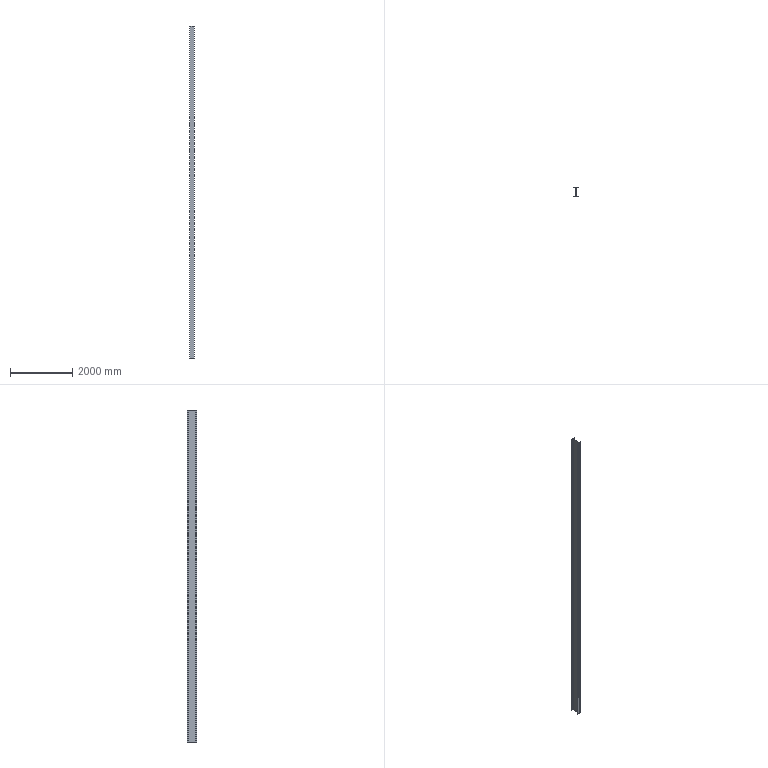Part | SolidWorks | features Extrusion 1 | 1 solid | 18 faces | box 150 x 300 x 10687 mm | volume 49994543 mm3 | plane 14 | cylinder 4 | commonest cylinder face diameters 26 x4
STEP:
#1=CARTESIAN_POINT('',(-75.,9.,0.));
#2=VERTEX_POINT('',#1);
#3=CARTESIAN_POINT('',(-75.,0.,0.));
#4=VERTEX_POINT('',#3);
#5=CARTESIAN_POINT('',(-75.,0.,0.));
#6=DIRECTION('',(0.,-1.,0.));
#7=VECTOR('',#6,1000.);
#8=LINE('',#5,#7);
#9=EDGE_CURVE('',#2,#4,#8,.T.);
#10=ORIENTED_EDGE('',*,*,#9,.T.);
#11=CARTESIAN_POINT('',(-75.,0.,10687.));
#12=VERTEX_POINT('',#11);
#13=CARTESIAN_POINT('',(-75.,0.,10687.));
#14=DIRECTION('',(0.,0.,-1.));
#15=VECTOR('',#14,1000.);
#16=LINE('',#13,#15);
#17=EDGE_CURVE('',#12,#4,#16,.T.);
#18=ORIENTED_EDGE('',*,*,#17,.F.);
#19=CARTESIAN_POINT('',(-75.,9.,10687.));
#20=VERTEX_POINT('',#19);
#21=CARTESIAN_POINT('',(-75.,0.,10687.));
#22=DIRECTION('',(0.,-1.,0.));
#23=VECTOR('',#22,1000.);
#24=LINE('',#21,#23);
#25=EDGE_CURVE('',#20,#12,#24,.T.);
#26=ORIENTED_EDGE('',*,*,#25,.F.);
#27=CARTESIAN_POINT('',(-75.,9.,10687.));
#28=DIRECTION('',(0.,0.,-1.));
#29=VECTOR('',#28,1000.);
#30=LINE('',#27,#29);
#31=EDGE_CURVE('',#20,#2,#30,.T.);
#32=ORIENTED_EDGE('',*,*,#31,.T.);
#33=EDGE_LOOP('',(#10,#18,#26,#32));
#34=FACE_OUTER_BOUND('',#33,.T.);
#35=CARTESIAN_POINT('',(-75.,0.,10687.));
#36=DIRECTION('',(1.,0.,0.));
#37=DIRECTION('',(0.,0.,-1.));
#38=AXIS2_PLACEMENT_3D('',#35,#36,#37);
#39=PLANE('',#38);
#40=ADVANCED_FACE('',(#34),#39,.F.);
#41=CARTESIAN_POINT('',(75.,0.,0.));
#42=VERTEX_POINT('',#41);
#43=CARTESIAN_POINT('',(75.,0.,0.));
#44=DIRECTION('',(1.,0.,0.));
#45=VECTOR('',#44,1000.);
#46=LINE('',#43,#45);
#47=EDGE_CURVE('',#4,#42,#46,.T.);
#48=ORIENTED_EDGE('',*,*,#47,.T.);
#49=CARTESIAN_POINT('',(75.,0.,10687.));
#50=VERTEX_POINT('',#49);
#51=CARTESIAN_POINT('',(75.,0.,10687.));
#52=DIRECTION('',(0.,0.,-1.));
#53=VECTOR('',#52,1000.);
#54=LINE('',#51,#53);
#55=EDGE_CURVE('',#50,#42,#54,.T.);
#56=ORIENTED_EDGE('',*,*,#55,.F.);
#57=CARTESIAN_POINT('',(75.,0.,10687.));
#58=DIRECTION('',(1.,0.,0.));
#59=VECTOR('',#58,1000.);
#60=LINE('',#57,#59);
#61=EDGE_CURVE('',#12,#50,#60,.T.);
#62=ORIENTED_EDGE('',*,*,#61,.F.);
#63=ORIENTED_EDGE('',*,*,#17,.T.);
#64=EDGE_LOOP('',(#48,#56,#62,#63));
#65=FACE_OUTER_BOUND('',#64,.T.);
#66=CARTESIAN_POINT('',(75.,0.,10687.));
#67=DIRECTION('',(0.,1.,0.));
#68=DIRECTION('',(-1.,0.,0.));
#69=AXIS2_PLACEMENT_3D('',#66,#67,#68);
#70=PLANE('',#69);
#71=ADVANCED_FACE('',(#65),#70,.F.);
#72=CARTESIAN_POINT('',(75.,9.,0.));
#73=VERTEX_POINT('',#72);
#74=CARTESIAN_POINT('',(75.,0.,0.));
#75=DIRECTION('',(0.,1.,0.));
#76=VECTOR('',#75,1000.);
#77=LINE('',#74,#76);
#78=EDGE_CURVE('',#42,#73,#77,.T.);
#79=ORIENTED_EDGE('',*,*,#78,.T.);
#80=CARTESIAN_POINT('',(75.,9.,10687.));
#81=VERTEX_POINT('',#80);
#82=CARTESIAN_POINT('',(75.,9.,10687.));
#83=DIRECTION('',(0.,0.,-1.));
#84=VECTOR('',#83,1000.);
#85=LINE('',#82,#84);
#86=EDGE_CURVE('',#81,#73,#85,.T.);
#87=ORIENTED_EDGE('',*,*,#86,.F.);
#88=CARTESIAN_POINT('',(75.,0.,10687.));
#89=DIRECTION('',(0.,1.,0.));
#90=VECTOR('',#89,1000.);
#91=LINE('',#88,#90);
#92=EDGE_CURVE('',#50,#81,#91,.T.);
#93=ORIENTED_EDGE('',*,*,#92,.F.);
#94=ORIENTED_EDGE('',*,*,#55,.T.);
#95=EDGE_LOOP('',(#79,#87,#93,#94));
#96=FACE_OUTER_BOUND('',#95,.T.);
#97=CARTESIAN_POINT('',(75.,0.,10687.));
#98=DIRECTION('',(-1.,0.,0.));
#99=DIRECTION('',(0.,0.,1.));
#100=AXIS2_PLACEMENT_3D('',#97,#98,#99);
#101=PLANE('',#100);
#102=ADVANCED_FACE('',(#96),#101,.F.);
#103=CARTESIAN_POINT('',(16.25,9.,0.));
#104=VERTEX_POINT('',#103);
#105=CARTESIAN_POINT('',(75.,9.,0.));
#106=DIRECTION('',(-1.,0.,0.));
#107=VECTOR('',#106,1000.);
#108=LINE('',#105,#107);
#109=EDGE_CURVE('',#73,#104,#108,.T.);
#110=ORIENTED_EDGE('',*,*,#109,.T.);
#111=CARTESIAN_POINT('',(16.25,9.,10687.));
#112=VERTEX_POINT('',#111);
#113=CARTESIAN_POINT('',(16.25,9.,10687.));
#114=DIRECTION('',(0.,0.,-1.));
#115=VECTOR('',#114,1000.);
#116=LINE('',#113,#115);
#117=EDGE_CURVE('',#112,#104,#116,.T.);
#118=ORIENTED_EDGE('',*,*,#117,.F.);
#119=CARTESIAN_POINT('',(75.,9.,10687.));
#120=DIRECTION('',(-1.,0.,0.));
#121=VECTOR('',#120,1000.);
#122=LINE('',#119,#121);
#123=EDGE_CURVE('',#81,#112,#122,.T.);
#124=ORIENTED_EDGE('',*,*,#123,.F.);
#125=ORIENTED_EDGE('',*,*,#86,.T.);
#126=EDGE_LOOP('',(#110,#118,#124,#125));
#127=FACE_OUTER_BOUND('',#126,.T.);
#128=CARTESIAN_POINT('',(75.,9.,10687.));
#129=DIRECTION('',(0.,-1.,0.));
#130=DIRECTION('',(1.,0.,0.));
#131=AXIS2_PLACEMENT_3D('',#128,#129,#130);
#132=PLANE('',#131);
#133=ADVANCED_FACE('',(#127),#132,.F.);
#134=CARTESIAN_POINT('',(3.25,22.,0.));
#135=VERTEX_POINT('',#134);
#136=CARTESIAN_POINT('',(16.25,22.,0.));
#137=DIRECTION('',(0.,0.,-1.));
#138=DIRECTION('',(-1.,0.,0.));
#139=AXIS2_PLACEMENT_3D('',#136,#137,#138);
#140=CIRCLE('',#139,13.);
#141=EDGE_CURVE('',#104,#135,#140,.T.);
#142=ORIENTED_EDGE('',*,*,#141,.T.);
#143=CARTESIAN_POINT('',(3.25,22.,10687.));
#144=VERTEX_POINT('',#143);
#145=CARTESIAN_POINT('',(3.25,22.,10687.));
#146=DIRECTION('',(0.,0.,-1.));
#147=VECTOR('',#146,1000.);
#148=LINE('',#145,#147);
#149=EDGE_CURVE('',#144,#135,#148,.T.);
#150=ORIENTED_EDGE('',*,*,#149,.F.);
#151=CARTESIAN_POINT('',(16.25,22.,10687.));
#152=DIRECTION('',(0.,0.,-1.));
#153=DIRECTION('',(-1.,0.,0.));
#154=AXIS2_PLACEMENT_3D('',#151,#152,#153);
#155=CIRCLE('',#154,13.);
#156=EDGE_CURVE('',#112,#144,#155,.T.);
#157=ORIENTED_EDGE('',*,*,#156,.F.);
#158=ORIENTED_EDGE('',*,*,#117,.T.);
#159=EDGE_LOOP('',(#142,#150,#157,#158));
#160=FACE_OUTER_BOUND('',#159,.T.);
#161=CARTESIAN_POINT('',(16.25,22.,10687.));
#162=DIRECTION('',(0.,0.,-1.));
#163=DIRECTION('',(-1.,0.,0.));
#164=AXIS2_PLACEMENT_3D('',#161,#162,#163);
#165=CYLINDRICAL_SURFACE('',#164,13.);
#166=ADVANCED_FACE('',(#160),#165,.F.);
#167=CARTESIAN_POINT('',(3.25,278.,0.));
#168=VERTEX_POINT('',#167);
#169=CARTESIAN_POINT('',(3.25,22.,0.));
#170=DIRECTION('',(0.,1.,0.));
#171=VECTOR('',#170,1000.);
#172=LINE('',#169,#171);
#173=EDGE_CURVE('',#135,#168,#172,.T.);
#174=ORIENTED_EDGE('',*,*,#173,.T.);
#175=CARTESIAN_POINT('',(3.25,278.,10687.));
#176=VERTEX_POINT('',#175);
#177=CARTESIAN_POINT('',(3.25,278.,10687.));
#178=DIRECTION('',(0.,0.,-1.));
#179=VECTOR('',#178,1000.);
#180=LINE('',#177,#179);
#181=EDGE_CURVE('',#176,#168,#180,.T.);
#182=ORIENTED_EDGE('',*,*,#181,.F.);
#183=CARTESIAN_POINT('',(3.25,22.,10687.));
#184=DIRECTION('',(0.,1.,0.));
#185=VECTOR('',#184,1000.);
#186=LINE('',#183,#185);
#187=EDGE_CURVE('',#144,#176,#186,.T.);
#188=ORIENTED_EDGE('',*,*,#187,.F.);
#189=ORIENTED_EDGE('',*,*,#149,.T.);
#190=EDGE_LOOP('',(#174,#182,#188,#189));
#191=FACE_OUTER_BOUND('',#190,.T.);
#192=CARTESIAN_POINT('',(3.25,22.,10687.));
#193=DIRECTION('',(-1.,0.,0.));
#194=DIRECTION('',(0.,0.,1.));
#195=AXIS2_PLACEMENT_3D('',#192,#193,#194);
#196=PLANE('',#195);
#197=ADVANCED_FACE('',(#191),#196,.F.);
#198=CARTESIAN_POINT('',(16.25,291.,0.));
#199=VERTEX_POINT('',#198);
#200=CARTESIAN_POINT('',(16.25,278.,0.));
#201=DIRECTION('',(0.,0.,-1.));
#202=DIRECTION('',(-1.,0.,0.));
#203=AXIS2_PLACEMENT_3D('',#200,#201,#202);
#204=CIRCLE('',#203,13.);
#205=EDGE_CURVE('',#168,#199,#204,.T.);
#206=ORIENTED_EDGE('',*,*,#205,.T.);
#207=CARTESIAN_POINT('',(16.25,291.,10687.));
#208=VERTEX_POINT('',#207);
#209=CARTESIAN_POINT('',(16.25,291.,10687.));
#210=DIRECTION('',(0.,0.,-1.));
#211=VECTOR('',#210,1000.);
#212=LINE('',#209,#211);
#213=EDGE_CURVE('',#208,#199,#212,.T.);
#214=ORIENTED_EDGE('',*,*,#213,.F.);
#215=CARTESIAN_POINT('',(16.25,278.,10687.));
#216=DIRECTION('',(0.,0.,-1.));
#217=DIRECTION('',(-1.,0.,0.));
#218=AXIS2_PLACEMENT_3D('',#215,#216,#217);
#219=CIRCLE('',#218,13.);
#220=EDGE_CURVE('',#176,#208,#219,.T.);
#221=ORIENTED_EDGE('',*,*,#220,.F.);
#222=ORIENTED_EDGE('',*,*,#181,.T.);
#223=EDGE_LOOP('',(#206,#214,#221,#222));
#224=FACE_OUTER_BOUND('',#223,.T.);
#225=CARTESIAN_POINT('',(16.25,278.,10687.));
#226=DIRECTION('',(0.,0.,-1.));
#227=DIRECTION('',(-1.,0.,0.));
#228=AXIS2_PLACEMENT_3D('',#225,#226,#227);
#229=CYLINDRICAL_SURFACE('',#228,13.);
#230=ADVANCED_FACE('',(#224),#229,.F.);
#231=CARTESIAN_POINT('',(75.,291.,0.));
#232=VERTEX_POINT('',#231);
#233=CARTESIAN_POINT('',(16.25,291.,0.));
#234=DIRECTION('',(1.,0.,0.));
#235=VECTOR('',#234,1000.);
#236=LINE('',#233,#235);
#237=EDGE_CURVE('',#199,#232,#236,.T.);
#238=ORIENTED_EDGE('',*,*,#237,.T.);
#239=CARTESIAN_POINT('',(75.,291.,10687.));
#240=VERTEX_POINT('',#239);
#241=CARTESIAN_POINT('',(75.,291.,10687.));
#242=DIRECTION('',(0.,0.,-1.));
#243=VECTOR('',#242,1000.);
#244=LINE('',#241,#243);
#245=EDGE_CURVE('',#240,#232,#244,.T.);
#246=ORIENTED_EDGE('',*,*,#245,.F.);
#247=CARTESIAN_POINT('',(16.25,291.,10687.));
#248=DIRECTION('',(1.,0.,0.));
#249=VECTOR('',#248,1000.);
#250=LINE('',#247,#249);
#251=EDGE_CURVE('',#208,#240,#250,.T.);
#252=ORIENTED_EDGE('',*,*,#251,.F.);
#253=ORIENTED_EDGE('',*,*,#213,.T.);
#254=EDGE_LOOP('',(#238,#246,#252,#253));
#255=FACE_OUTER_BOUND('',#254,.T.);
#256=CARTESIAN_POINT('',(16.25,291.,10687.));
#257=DIRECTION('',(0.,1.,0.));
#258=DIRECTION('',(-1.,0.,0.));
#259=AXIS2_PLACEMENT_3D('',#256,#257,#258);
#260=PLANE('',#259);
#261=ADVANCED_FACE('',(#255),#260,.F.);
#262=CARTESIAN_POINT('',(75.,300.,0.));
#263=VERTEX_POINT('',#262);
#264=CARTESIAN_POINT('',(75.,291.,0.));
#265=DIRECTION('',(0.,1.,0.));
#266=VECTOR('',#265,1000.);
#267=LINE('',#264,#266);
#268=EDGE_CURVE('',#232,#263,#267,.T.);
#269=ORIENTED_EDGE('',*,*,#268,.T.);
#270=CARTESIAN_POINT('',(75.,300.,10687.));
#271=VERTEX_POINT('',#270);
#272=CARTESIAN_POINT('',(75.,300.,10687.));
#273=DIRECTION('',(0.,0.,-1.));
#274=VECTOR('',#273,1000.);
#275=LINE('',#272,#274);
#276=EDGE_CURVE('',#271,#263,#275,.T.);
#277=ORIENTED_EDGE('',*,*,#276,.F.);
#278=CARTESIAN_POINT('',(75.,291.,10687.));
#279=DIRECTION('',(0.,1.,0.));
#280=VECTOR('',#279,1000.);
#281=LINE('',#278,#280);
#282=EDGE_CURVE('',#240,#271,#281,.T.);
#283=ORIENTED_EDGE('',*,*,#282,.F.);
#284=ORIENTED_EDGE('',*,*,#245,.T.);
#285=EDGE_LOOP('',(#269,#277,#283,#284));
#286=FACE_OUTER_BOUND('',#285,.T.);
#287=CARTESIAN_POINT('',(75.,291.,10687.));
#288=DIRECTION('',(-1.,0.,0.));
#289=DIRECTION('',(0.,-1.,0.));
#290=AXIS2_PLACEMENT_3D('',#287,#288,#289);
#291=PLANE('',#290);
#292=ADVANCED_FACE('',(#286),#291,.F.);
#293=CARTESIAN_POINT('',(-75.,300.,0.));
#294=VERTEX_POINT('',#293);
#295=CARTESIAN_POINT('',(-75.,300.,0.));
#296=DIRECTION('',(-1.,0.,0.));
#297=VECTOR('',#296,1000.);
#298=LINE('',#295,#297);
#299=EDGE_CURVE('',#263,#294,#298,.T.);
#300=ORIENTED_EDGE('',*,*,#299,.T.);
#301=CARTESIAN_POINT('',(-75.,300.,10687.));
#302=VERTEX_POINT('',#301);
#303=CARTESIAN_POINT('',(-75.,300.,10687.));
#304=DIRECTION('',(0.,0.,-1.));
#305=VECTOR('',#304,1000.);
#306=LINE('',#303,#305);
#307=EDGE_CURVE('',#302,#294,#306,.T.);
#308=ORIENTED_EDGE('',*,*,#307,.F.);
#309=CARTESIAN_POINT('',(-75.,300.,10687.));
#310=DIRECTION('',(-1.,0.,0.));
#311=VECTOR('',#310,1000.);
#312=LINE('',#309,#311);
#313=EDGE_CURVE('',#271,#302,#312,.T.);
#314=ORIENTED_EDGE('',*,*,#313,.F.);
#315=ORIENTED_EDGE('',*,*,#276,.T.);
#316=EDGE_LOOP('',(#300,#308,#314,#315));
#317=FACE_OUTER_BOUND('',#316,.T.);
#318=CARTESIAN_POINT('',(-75.,300.,10687.));
#319=DIRECTION('',(0.,-1.,0.));
#320=DIRECTION('',(0.,0.,-1.));
#321=AXIS2_PLACEMENT_3D('',#318,#319,#320);
#322=PLANE('',#321);
#323=ADVANCED_FACE('',(#317),#322,.F.);
#324=CARTESIAN_POINT('',(-75.,291.,0.));
#325=VERTEX_POINT('',#324);
#326=CARTESIAN_POINT('',(-75.,291.,0.));
#327=DIRECTION('',(0.,-1.,0.));
#328=VECTOR('',#327,1000.);
#329=LINE('',#326,#328);
#330=EDGE_CURVE('',#294,#325,#329,.T.);
#331=ORIENTED_EDGE('',*,*,#330,.T.);
#332=CARTESIAN_POINT('',(-75.,291.,10687.));
#333=VERTEX_POINT('',#332);
#334=CARTESIAN_POINT('',(-75.,291.,10687.));
#335=DIRECTION('',(0.,0.,-1.));
#336=VECTOR('',#335,1000.);
#337=LINE('',#334,#336);
#338=EDGE_CURVE('',#333,#325,#337,.T.);
#339=ORIENTED_EDGE('',*,*,#338,.F.);
#340=CARTESIAN_POINT('',(-75.,291.,10687.));
#341=DIRECTION('',(0.,-1.,0.));
#342=VECTOR('',#341,1000.);
#343=LINE('',#340,#342);
#344=EDGE_CURVE('',#302,#333,#343,.T.);
#345=ORIENTED_EDGE('',*,*,#344,.F.);
#346=ORIENTED_EDGE('',*,*,#307,.T.);
#347=EDGE_LOOP('',(#331,#339,#345,#346));
#348=FACE_OUTER_BOUND('',#347,.T.);
#349=CARTESIAN_POINT('',(-75.,291.,10687.));
#350=DIRECTION('',(1.,0.,0.));
#351=DIRECTION('',(0.,1.,0.));
#352=AXIS2_PLACEMENT_3D('',#349,#350,#351);
#353=PLANE('',#352);
#354=ADVANCED_FACE('',(#348),#353,.F.);
#355=CARTESIAN_POINT('',(-16.25,291.,0.));
#356=VERTEX_POINT('',#355);
#357=CARTESIAN_POINT('',(-16.25,291.,0.));
#358=DIRECTION('',(1.,0.,0.));
#359=VECTOR('',#358,1000.);
#360=LINE('',#357,#359);
#361=EDGE_CURVE('',#325,#356,#360,.T.);
#362=ORIENTED_EDGE('',*,*,#361,.T.);
#363=CARTESIAN_POINT('',(-16.25,291.,10687.));
#364=VERTEX_POINT('',#363);
#365=CARTESIAN_POINT('',(-16.25,291.,10687.));
#366=DIRECTION('',(0.,0.,-1.));
#367=VECTOR('',#366,1000.);
#368=LINE('',#365,#367);
#369=EDGE_CURVE('',#364,#356,#368,.T.);
#370=ORIENTED_EDGE('',*,*,#369,.F.);
#371=CARTESIAN_POINT('',(-16.25,291.,10687.));
#372=DIRECTION('',(1.,0.,0.));
#373=VECTOR('',#372,1000.);
#374=LINE('',#371,#373);
#375=EDGE_CURVE('',#333,#364,#374,.T.);
#376=ORIENTED_EDGE('',*,*,#375,.F.);
#377=ORIENTED_EDGE('',*,*,#338,.T.);
#378=EDGE_LOOP('',(#362,#370,#376,#377));
#379=FACE_OUTER_BOUND('',#378,.T.);
#380=CARTESIAN_POINT('',(-16.25,291.,10687.));
#381=DIRECTION('',(0.,1.,0.));
#382=DIRECTION('',(-1.,0.,0.));
#383=AXIS2_PLACEMENT_3D('',#380,#381,#382);
#384=PLANE('',#383);
#385=ADVANCED_FACE('',(#379),#384,.F.);
#386=CARTESIAN_POINT('',(-3.25,278.,0.));
#387=VERTEX_POINT('',#386);
#388=CARTESIAN_POINT('',(-16.25,278.,0.));
#389=DIRECTION('',(0.,0.,-1.));
#390=DIRECTION('',(1.,0.,0.));
#391=AXIS2_PLACEMENT_3D('',#388,#389,#390);
#392=CIRCLE('',#391,13.);
#393=EDGE_CURVE('',#356,#387,#392,.T.);
#394=ORIENTED_EDGE('',*,*,#393,.T.);
#395=CARTESIAN_POINT('',(-3.25,278.,10687.));
#396=VERTEX_POINT('',#395);
#397=CARTESIAN_POINT('',(-3.25,278.,10687.));
#398=DIRECTION('',(0.,0.,-1.));
#399=VECTOR('',#398,1000.);
#400=LINE('',#397,#399);
#401=EDGE_CURVE('',#396,#387,#400,.T.);
#402=ORIENTED_EDGE('',*,*,#401,.F.);
#403=CARTESIAN_POINT('',(-16.25,278.,10687.));
#404=DIRECTION('',(0.,0.,-1.));
#405=DIRECTION('',(1.,0.,0.));
#406=AXIS2_PLACEMENT_3D('',#403,#404,#405);
#407=CIRCLE('',#406,13.);
#408=EDGE_CURVE('',#364,#396,#407,.T.);
#409=ORIENTED_EDGE('',*,*,#408,.F.);
#410=ORIENTED_EDGE('',*,*,#369,.T.);
#411=EDGE_LOOP('',(#394,#402,#409,#410));
#412=FACE_OUTER_BOUND('',#411,.T.);
#413=CARTESIAN_POINT('',(-16.25,278.,10687.));
#414=DIRECTION('',(0.,0.,-1.));
#415=DIRECTION('',(-1.,0.,0.));
#416=AXIS2_PLACEMENT_3D('',#413,#414,#415);
#417=CYLINDRICAL_SURFACE('',#416,13.);
#418=ADVANCED_FACE('',(#412),#417,.F.);
#419=CARTESIAN_POINT('',(-3.25,22.,0.));
#420=VERTEX_POINT('',#419);
#421=CARTESIAN_POINT('',(-3.25,22.,0.));
#422=DIRECTION('',(0.,-1.,0.));
#423=VECTOR('',#422,1000.);
#424=LINE('',#421,#423);
#425=EDGE_CURVE('',#387,#420,#424,.T.);
#426=ORIENTED_EDGE('',*,*,#425,.T.);
#427=CARTESIAN_POINT('',(-3.25,22.,10687.));
#428=VERTEX_POINT('',#427);
#429=CARTESIAN_POINT('',(-3.25,22.,10687.));
#430=DIRECTION('',(0.,0.,-1.));
#431=VECTOR('',#430,1000.);
#432=LINE('',#429,#431);
#433=EDGE_CURVE('',#428,#420,#432,.T.);
#434=ORIENTED_EDGE('',*,*,#433,.F.);
#435=CARTESIAN_POINT('',(-3.25,22.,10687.));
#436=DIRECTION('',(0.,-1.,0.));
#437=VECTOR('',#436,1000.);
#438=LINE('',#435,#437);
#439=EDGE_CURVE('',#396,#428,#438,.T.);
#440=ORIENTED_EDGE('',*,*,#439,.F.);
#441=ORIENTED_EDGE('',*,*,#401,.T.);
#442=EDGE_LOOP('',(#426,#434,#440,#441));
#443=FACE_OUTER_BOUND('',#442,.T.);
#444=CARTESIAN_POINT('',(-3.25,22.,10687.));
#445=DIRECTION('',(1.,0.,0.));
#446=DIRECTION('',(0.,0.,-1.));
#447=AXIS2_PLACEMENT_3D('',#444,#445,#446);
#448=PLANE('',#447);
#449=ADVANCED_FACE('',(#443),#448,.F.);
#450=CARTESIAN_POINT('',(-16.25,9.,0.));
#451=VERTEX_POINT('',#450);
#452=CARTESIAN_POINT('',(-16.25,22.,0.));
#453=DIRECTION('',(0.,0.,-1.));
#454=DIRECTION('',(-1.,0.,0.));
#455=AXIS2_PLACEMENT_3D('',#452,#453,#454);
#456=CIRCLE('',#455,13.);
#457=EDGE_CURVE('',#420,#451,#456,.T.);
#458=ORIENTED_EDGE('',*,*,#457,.T.);
#459=CARTESIAN_POINT('',(-16.25,9.,10687.));
#460=VERTEX_POINT('',#459);
#461=CARTESIAN_POINT('',(-16.25,9.,10687.));
#462=DIRECTION('',(0.,0.,-1.));
#463=VECTOR('',#462,1000.);
#464=LINE('',#461,#463);
#465=EDGE_CURVE('',#460,#451,#464,.T.);
#466=ORIENTED_EDGE('',*,*,#465,.F.);
#467=CARTESIAN_POINT('',(-16.25,22.,10687.));
#468=DIRECTION('',(0.,0.,-1.));
#469=DIRECTION('',(-1.,0.,0.));
#470=AXIS2_PLACEMENT_3D('',#467,#468,#469);
#471=CIRCLE('',#470,13.);
#472=EDGE_CURVE('',#428,#460,#471,.T.);
#473=ORIENTED_EDGE('',*,*,#472,.F.);
#474=ORIENTED_EDGE('',*,*,#433,.T.);
#475=EDGE_LOOP('',(#458,#466,#473,#474));
#476=FACE_OUTER_BOUND('',#475,.T.);
#477=CARTESIAN_POINT('',(-16.25,22.,10687.));
#478=DIRECTION('',(0.,0.,-1.));
#479=DIRECTION('',(-1.,0.,0.));
#480=AXIS2_PLACEMENT_3D('',#477,#478,#479);
#481=CYLINDRICAL_SURFACE('',#480,13.);
#482=ADVANCED_FACE('',(#476),#481,.F.);
#483=CARTESIAN_POINT('',(-75.,9.,0.));
#484=DIRECTION('',(-1.,0.,0.));
#485=VECTOR('',#484,1000.);
#486=LINE('',#483,#485);
#487=EDGE_CURVE('',#451,#2,#486,.T.);
#488=ORIENTED_EDGE('',*,*,#487,.T.);
#489=ORIENTED_EDGE('',*,*,#31,.F.);
#490=CARTESIAN_POINT('',(-75.,9.,10687.));
#491=DIRECTION('',(-1.,0.,0.));
#492=VECTOR('',#491,1000.);
#493=LINE('',#490,#492);
#494=EDGE_CURVE('',#460,#20,#493,.T.);
#495=ORIENTED_EDGE('',*,*,#494,.F.);
#496=ORIENTED_EDGE('',*,*,#465,.T.);
#497=EDGE_LOOP('',(#488,#489,#495,#496));
#498=FACE_OUTER_BOUND('',#497,.T.);
#499=CARTESIAN_POINT('',(-75.,9.,10687.));
#500=DIRECTION('',(0.,-1.,0.));
#501=DIRECTION('',(1.,0.,0.));
#502=AXIS2_PLACEMENT_3D('',#499,#500,#501);
#503=PLANE('',#502);
#504=ADVANCED_FACE('',(#498),#503,.F.);
#505=ORIENTED_EDGE('',*,*,#25,.T.);
#506=ORIENTED_EDGE('',*,*,#61,.T.);
#507=ORIENTED_EDGE('',*,*,#92,.T.);
#508=ORIENTED_EDGE('',*,*,#123,.T.);
#509=ORIENTED_EDGE('',*,*,#156,.T.);
#510=ORIENTED_EDGE('',*,*,#187,.T.);
#511=ORIENTED_EDGE('',*,*,#220,.T.);
#512=ORIENTED_EDGE('',*,*,#251,.T.);
#513=ORIENTED_EDGE('',*,*,#282,.T.);
#514=ORIENTED_EDGE('',*,*,#313,.T.);
#515=ORIENTED_EDGE('',*,*,#344,.T.);
#516=ORIENTED_EDGE('',*,*,#375,.T.);
#517=ORIENTED_EDGE('',*,*,#408,.T.);
#518=ORIENTED_EDGE('',*,*,#439,.T.);
#519=ORIENTED_EDGE('',*,*,#472,.T.);
#520=ORIENTED_EDGE('',*,*,#494,.T.);
#521=EDGE_LOOP('',(#505,#506,#507,#508,#509,#510,#511,#512,#513,#514,#515,#516,#517,#518,#519,#520));
#522=FACE_OUTER_BOUND('',#521,.T.);
#523=CARTESIAN_POINT('',(-16.25,22.,10687.));
#524=DIRECTION('',(0.,0.,-1.));
#525=DIRECTION('',(-1.,0.,0.));
#526=AXIS2_PLACEMENT_3D('',#523,#524,#525);
#527=PLANE('',#526);
#528=ADVANCED_FACE('',(#522),#527,.F.);
#529=ORIENTED_EDGE('',*,*,#9,.F.);
#530=ORIENTED_EDGE('',*,*,#487,.F.);
#531=ORIENTED_EDGE('',*,*,#457,.F.);
#532=ORIENTED_EDGE('',*,*,#425,.F.);
#533=ORIENTED_EDGE('',*,*,#393,.F.);
#534=ORIENTED_EDGE('',*,*,#361,.F.);
#535=ORIENTED_EDGE('',*,*,#330,.F.);
#536=ORIENTED_EDGE('',*,*,#299,.F.);
#537=ORIENTED_EDGE('',*,*,#268,.F.);
#538=ORIENTED_EDGE('',*,*,#237,.F.);
#539=ORIENTED_EDGE('',*,*,#205,.F.);
#540=ORIENTED_EDGE('',*,*,#173,.F.);
#541=ORIENTED_EDGE('',*,*,#141,.F.);
#542=ORIENTED_EDGE('',*,*,#109,.F.);
#543=ORIENTED_EDGE('',*,*,#78,.F.);
#544=ORIENTED_EDGE('',*,*,#47,.F.);
#545=EDGE_LOOP('',(#529,#530,#531,#532,#533,#534,#535,#536,#537,#538,#539,#540,#541,#542,#543,#544));
#546=FACE_OUTER_BOUND('',#545,.T.);
#547=CARTESIAN_POINT('',(-16.25,22.,0.));
#548=DIRECTION('',(0.,0.,-1.));
#549=DIRECTION('',(-1.,0.,0.));
#550=AXIS2_PLACEMENT_3D('',#547,#548,#549);
#551=PLANE('',#550);
#552=ADVANCED_FACE('',(#546),#551,.T.);
#553=CLOSED_SHELL('',(#40,#71,#102,#133,#166,#197,#230,#261,#292,#323,#354,#385,#418,#449,#482,#504,#528,#552));
#554=MANIFOLD_SOLID_BREP('',#553);
#555=CARTESIAN_POINT('',(0.,0.,0.));
#556=DIRECTION('',(0.,0.,1.));
#557=DIRECTION('',(1.,0.,0.));
#558=AXIS2_PLACEMENT_3D('',#555,#556,#557);
#559=(LENGTH_UNIT()NAMED_UNIT(*)SI_UNIT(.MILLI.,.METRE.));
#560=UNCERTAINTY_MEASURE_WITH_UNIT(LENGTH_MEASURE(0.00001),#559,'','');
#561=(NAMED_UNIT(*)PLANE_ANGLE_UNIT()SI_UNIT($,.RADIAN.));
#562=(NAMED_UNIT(*)SI_UNIT($,.STERADIAN.)SOLID_ANGLE_UNIT());
#563=(GEOMETRIC_REPRESENTATION_CONTEXT(3)GLOBAL_UNCERTAINTY_ASSIGNED_CONTEXT((#560))GLOBAL_UNIT_ASSIGNED_CONTEXT((#559,#561,#562))REPRESENTATION_CONTEXT('',''));
#564=ADVANCED_BREP_SHAPE_REPRESENTATION('',(#554,#558),#563);